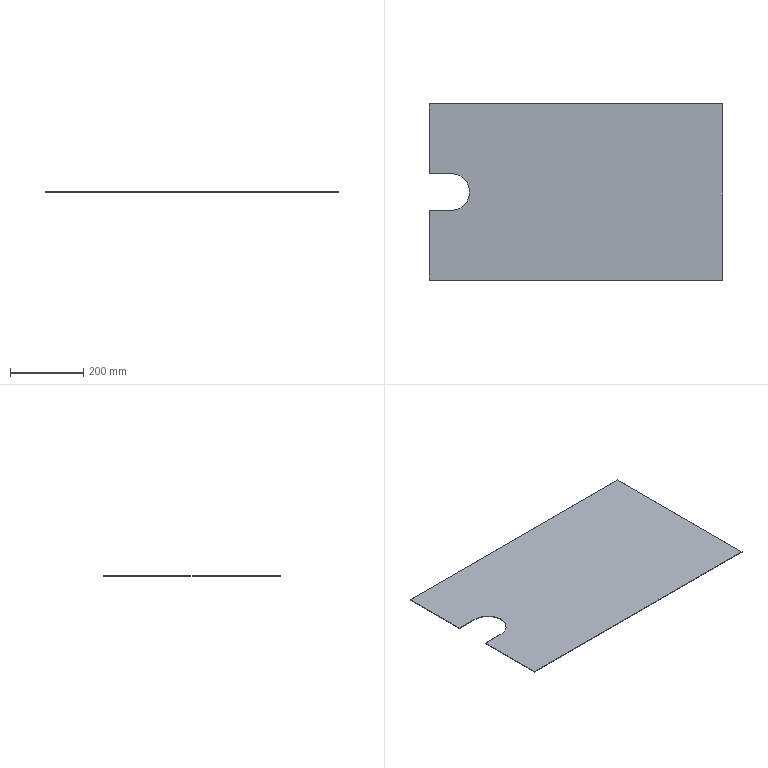Part | SolidWorks | features FlatPattern 1, ICE 1, SMBaseFlange 1, SheetMetal 1 | 1 solid | 10 faces | box 800 x 480 x 1.5 mm | volume 561110 mm3 | plane 9 | cylinder 1 | commonest cylinder face diameters 100 x1
STEP:
#1=CARTESIAN_POINT('',(-585.,-50.,-1.5));
#2=VERTEX_POINT('',#1);
#3=CARTESIAN_POINT('',(-585.,-50.,0.));
#4=VERTEX_POINT('',#3);
#5=CARTESIAN_POINT('',(-585.,-50.,-1.5));
#6=DIRECTION('',(0.,0.,1.));
#7=VECTOR('',#6,1000.);
#8=LINE('',#5,#7);
#9=EDGE_CURVE('',#2,#4,#8,.T.);
#10=ORIENTED_EDGE('',*,*,#9,.F.);
#11=CARTESIAN_POINT('',(-585.,-240.,-1.5));
#12=VERTEX_POINT('',#11);
#13=CARTESIAN_POINT('',(-585.,240.,-1.5));
#14=DIRECTION('',(0.,-1.,0.));
#15=VECTOR('',#14,1000.);
#16=LINE('',#13,#15);
#17=EDGE_CURVE('',#2,#12,#16,.T.);
#18=ORIENTED_EDGE('',*,*,#17,.T.);
#19=CARTESIAN_POINT('',(-585.,-240.,0.));
#20=VERTEX_POINT('',#19);
#21=CARTESIAN_POINT('',(-585.,-240.,-1.5));
#22=DIRECTION('',(0.,0.,1.));
#23=VECTOR('',#22,1000.);
#24=LINE('',#21,#23);
#25=EDGE_CURVE('',#12,#20,#24,.T.);
#26=ORIENTED_EDGE('',*,*,#25,.T.);
#27=CARTESIAN_POINT('',(-585.,240.,0.));
#28=DIRECTION('',(0.,-1.,0.));
#29=VECTOR('',#28,1000.);
#30=LINE('',#27,#29);
#31=EDGE_CURVE('',#4,#20,#30,.T.);
#32=ORIENTED_EDGE('',*,*,#31,.F.);
#33=EDGE_LOOP('',(#10,#18,#26,#32));
#34=FACE_OUTER_BOUND('',#33,.T.);
#35=CARTESIAN_POINT('',(-585.,240.,-1.5));
#36=DIRECTION('',(-1.,0.,0.));
#37=DIRECTION('',(0.,0.,1.));
#38=AXIS2_PLACEMENT_3D('',#35,#36,#37);
#39=PLANE('',#38);
#40=ADVANCED_FACE('',(#34),#39,.T.);
#41=CARTESIAN_POINT('',(215.,-240.,0.));
#42=VERTEX_POINT('',#41);
#43=CARTESIAN_POINT('',(215.,240.,0.));
#44=VERTEX_POINT('',#43);
#45=CARTESIAN_POINT('',(215.,240.,0.));
#46=DIRECTION('',(0.,1.,0.));
#47=VECTOR('',#46,1000.);
#48=LINE('',#45,#47);
#49=EDGE_CURVE('',#42,#44,#48,.T.);
#50=ORIENTED_EDGE('',*,*,#49,.F.);
#51=CARTESIAN_POINT('',(215.,-240.,-1.5));
#52=VERTEX_POINT('',#51);
#53=CARTESIAN_POINT('',(215.,-240.,-1.5));
#54=DIRECTION('',(0.,0.,1.));
#55=VECTOR('',#54,1000.);
#56=LINE('',#53,#55);
#57=EDGE_CURVE('',#52,#42,#56,.T.);
#58=ORIENTED_EDGE('',*,*,#57,.F.);
#59=CARTESIAN_POINT('',(215.,240.,-1.5));
#60=VERTEX_POINT('',#59);
#61=CARTESIAN_POINT('',(215.,240.,-1.5));
#62=DIRECTION('',(0.,1.,0.));
#63=VECTOR('',#62,1000.);
#64=LINE('',#61,#63);
#65=EDGE_CURVE('',#52,#60,#64,.T.);
#66=ORIENTED_EDGE('',*,*,#65,.T.);
#67=CARTESIAN_POINT('',(215.,240.,-1.5));
#68=DIRECTION('',(0.,0.,1.));
#69=VECTOR('',#68,1000.);
#70=LINE('',#67,#69);
#71=EDGE_CURVE('',#60,#44,#70,.T.);
#72=ORIENTED_EDGE('',*,*,#71,.T.);
#73=EDGE_LOOP('',(#50,#58,#66,#72));
#74=FACE_OUTER_BOUND('',#73,.T.);
#75=CARTESIAN_POINT('',(215.,240.,-1.5));
#76=DIRECTION('',(1.,0.,0.));
#77=DIRECTION('',(0.,0.,-1.));
#78=AXIS2_PLACEMENT_3D('',#75,#76,#77);
#79=PLANE('',#78);
#80=ADVANCED_FACE('',(#74),#79,.T.);
#81=CARTESIAN_POINT('',(-585.,-240.,0.));
#82=DIRECTION('',(1.,0.,0.));
#83=VECTOR('',#82,1000.);
#84=LINE('',#81,#83);
#85=EDGE_CURVE('',#20,#42,#84,.T.);
#86=ORIENTED_EDGE('',*,*,#85,.F.);
#87=ORIENTED_EDGE('',*,*,#25,.F.);
#88=CARTESIAN_POINT('',(-585.,-240.,-1.5));
#89=DIRECTION('',(1.,0.,0.));
#90=VECTOR('',#89,1000.);
#91=LINE('',#88,#90);
#92=EDGE_CURVE('',#12,#52,#91,.T.);
#93=ORIENTED_EDGE('',*,*,#92,.T.);
#94=ORIENTED_EDGE('',*,*,#57,.T.);
#95=EDGE_LOOP('',(#86,#87,#93,#94));
#96=FACE_OUTER_BOUND('',#95,.T.);
#97=CARTESIAN_POINT('',(-585.,-240.,-1.5));
#98=DIRECTION('',(0.,-1.,0.));
#99=DIRECTION('',(0.,0.,-1.));
#100=AXIS2_PLACEMENT_3D('',#97,#98,#99);
#101=PLANE('',#100);
#102=ADVANCED_FACE('',(#96),#101,.T.);
#103=CARTESIAN_POINT('',(-585.,50.,0.));
#104=VERTEX_POINT('',#103);
#105=CARTESIAN_POINT('',(-585.,50.,-1.5));
#106=VERTEX_POINT('',#105);
#107=CARTESIAN_POINT('',(-585.,50.,-1.5));
#108=DIRECTION('',(0.,0.,-1.));
#109=VECTOR('',#108,1000.);
#110=LINE('',#107,#109);
#111=EDGE_CURVE('',#104,#106,#110,.T.);
#112=ORIENTED_EDGE('',*,*,#111,.F.);
#113=CARTESIAN_POINT('',(-585.,240.,0.));
#114=VERTEX_POINT('',#113);
#115=CARTESIAN_POINT('',(-585.,240.,0.));
#116=DIRECTION('',(0.,-1.,0.));
#117=VECTOR('',#116,1000.);
#118=LINE('',#115,#117);
#119=EDGE_CURVE('',#114,#104,#118,.T.);
#120=ORIENTED_EDGE('',*,*,#119,.F.);
#121=CARTESIAN_POINT('',(-585.,240.,-1.5));
#122=VERTEX_POINT('',#121);
#123=CARTESIAN_POINT('',(-585.,240.,-1.5));
#124=DIRECTION('',(0.,0.,1.));
#125=VECTOR('',#124,1000.);
#126=LINE('',#123,#125);
#127=EDGE_CURVE('',#122,#114,#126,.T.);
#128=ORIENTED_EDGE('',*,*,#127,.F.);
#129=CARTESIAN_POINT('',(-585.,240.,-1.5));
#130=DIRECTION('',(0.,-1.,0.));
#131=VECTOR('',#130,1000.);
#132=LINE('',#129,#131);
#133=EDGE_CURVE('',#122,#106,#132,.T.);
#134=ORIENTED_EDGE('',*,*,#133,.T.);
#135=EDGE_LOOP('',(#112,#120,#128,#134));
#136=FACE_OUTER_BOUND('',#135,.T.);
#137=CARTESIAN_POINT('',(-585.,240.,-1.5));
#138=DIRECTION('',(-1.,0.,0.));
#139=DIRECTION('',(0.,0.,1.));
#140=AXIS2_PLACEMENT_3D('',#137,#138,#139);
#141=PLANE('',#140);
#142=ADVANCED_FACE('',(#136),#141,.T.);
#143=CARTESIAN_POINT('',(-585.,240.,0.));
#144=DIRECTION('',(-1.,0.,0.));
#145=VECTOR('',#144,1000.);
#146=LINE('',#143,#145);
#147=EDGE_CURVE('',#44,#114,#146,.T.);
#148=ORIENTED_EDGE('',*,*,#147,.F.);
#149=ORIENTED_EDGE('',*,*,#71,.F.);
#150=CARTESIAN_POINT('',(-585.,240.,-1.5));
#151=DIRECTION('',(-1.,0.,0.));
#152=VECTOR('',#151,1000.);
#153=LINE('',#150,#152);
#154=EDGE_CURVE('',#60,#122,#153,.T.);
#155=ORIENTED_EDGE('',*,*,#154,.T.);
#156=ORIENTED_EDGE('',*,*,#127,.T.);
#157=EDGE_LOOP('',(#148,#149,#155,#156));
#158=FACE_OUTER_BOUND('',#157,.T.);
#159=CARTESIAN_POINT('',(-585.,240.,-1.5));
#160=DIRECTION('',(0.,1.,0.));
#161=DIRECTION('',(0.,0.,1.));
#162=AXIS2_PLACEMENT_3D('',#159,#160,#161);
#163=PLANE('',#162);
#164=ADVANCED_FACE('',(#158),#163,.T.);
#165=ORIENTED_EDGE('',*,*,#17,.F.);
#166=CARTESIAN_POINT('',(-525.,-50.,-1.5));
#167=VERTEX_POINT('',#166);
#168=CARTESIAN_POINT('',(0.,-50.,-1.5));
#169=DIRECTION('',(1.,0.,0.));
#170=VECTOR('',#169,1000.);
#171=LINE('',#168,#170);
#172=EDGE_CURVE('',#2,#167,#171,.T.);
#173=ORIENTED_EDGE('',*,*,#172,.T.);
#174=CARTESIAN_POINT('',(-525.,50.,-1.5));
#175=VERTEX_POINT('',#174);
#176=CARTESIAN_POINT('',(-525.,0.,-1.5));
#177=DIRECTION('',(0.,0.,1.));
#178=DIRECTION('',(1.,0.,0.));
#179=AXIS2_PLACEMENT_3D('',#176,#177,#178);
#180=CIRCLE('',#179,50.);
#181=EDGE_CURVE('',#167,#175,#180,.T.);
#182=ORIENTED_EDGE('',*,*,#181,.T.);
#183=CARTESIAN_POINT('',(0.,50.,-1.5));
#184=DIRECTION('',(-1.,0.,0.));
#185=VECTOR('',#184,1000.);
#186=LINE('',#183,#185);
#187=EDGE_CURVE('',#175,#106,#186,.T.);
#188=ORIENTED_EDGE('',*,*,#187,.T.);
#189=ORIENTED_EDGE('',*,*,#133,.F.);
#190=ORIENTED_EDGE('',*,*,#154,.F.);
#191=ORIENTED_EDGE('',*,*,#65,.F.);
#192=ORIENTED_EDGE('',*,*,#92,.F.);
#193=EDGE_LOOP('',(#165,#173,#182,#188,#189,#190,#191,#192));
#194=FACE_OUTER_BOUND('',#193,.T.);
#195=CARTESIAN_POINT('',(0.,0.,-1.5));
#196=DIRECTION('',(0.,0.,1.));
#197=DIRECTION('',(1.,0.,0.));
#198=AXIS2_PLACEMENT_3D('',#195,#196,#197);
#199=PLANE('',#198);
#200=ADVANCED_FACE('',(#194),#199,.F.);
#201=CARTESIAN_POINT('',(-525.,-50.,0.));
#202=VERTEX_POINT('',#201);
#203=CARTESIAN_POINT('',(0.,-50.,0.));
#204=DIRECTION('',(1.,0.,0.));
#205=VECTOR('',#204,1000.);
#206=LINE('',#203,#205);
#207=EDGE_CURVE('',#4,#202,#206,.T.);
#208=ORIENTED_EDGE('',*,*,#207,.F.);
#209=ORIENTED_EDGE('',*,*,#31,.T.);
#210=ORIENTED_EDGE('',*,*,#85,.T.);
#211=ORIENTED_EDGE('',*,*,#49,.T.);
#212=ORIENTED_EDGE('',*,*,#147,.T.);
#213=ORIENTED_EDGE('',*,*,#119,.T.);
#214=CARTESIAN_POINT('',(-525.,50.,0.));
#215=VERTEX_POINT('',#214);
#216=CARTESIAN_POINT('',(0.,50.,0.));
#217=DIRECTION('',(-1.,0.,0.));
#218=VECTOR('',#217,1000.);
#219=LINE('',#216,#218);
#220=EDGE_CURVE('',#215,#104,#219,.T.);
#221=ORIENTED_EDGE('',*,*,#220,.F.);
#222=CARTESIAN_POINT('',(-525.,0.,0.));
#223=DIRECTION('',(0.,0.,1.));
#224=DIRECTION('',(1.,0.,0.));
#225=AXIS2_PLACEMENT_3D('',#222,#223,#224);
#226=CIRCLE('',#225,50.);
#227=EDGE_CURVE('',#202,#215,#226,.T.);
#228=ORIENTED_EDGE('',*,*,#227,.F.);
#229=EDGE_LOOP('',(#208,#209,#210,#211,#212,#213,#221,#228));
#230=FACE_OUTER_BOUND('',#229,.T.);
#231=CARTESIAN_POINT('',(0.,0.,0.));
#232=DIRECTION('',(0.,0.,1.));
#233=DIRECTION('',(1.,0.,0.));
#234=AXIS2_PLACEMENT_3D('',#231,#232,#233);
#235=PLANE('',#234);
#236=ADVANCED_FACE('',(#230),#235,.T.);
#237=ORIENTED_EDGE('',*,*,#9,.T.);
#238=ORIENTED_EDGE('',*,*,#207,.T.);
#239=CARTESIAN_POINT('',(-525.,-50.,0.5));
#240=DIRECTION('',(0.,0.,-1.));
#241=VECTOR('',#240,1000.);
#242=LINE('',#239,#241);
#243=EDGE_CURVE('',#202,#167,#242,.T.);
#244=ORIENTED_EDGE('',*,*,#243,.T.);
#245=ORIENTED_EDGE('',*,*,#172,.F.);
#246=EDGE_LOOP('',(#237,#238,#244,#245));
#247=FACE_OUTER_BOUND('',#246,.T.);
#248=CARTESIAN_POINT('',(-525.,-50.,0.5));
#249=DIRECTION('',(0.,-1.,0.));
#250=DIRECTION('',(0.,0.,-1.));
#251=AXIS2_PLACEMENT_3D('',#248,#249,#250);
#252=PLANE('',#251);
#253=ADVANCED_FACE('',(#247),#252,.F.);
#254=ORIENTED_EDGE('',*,*,#243,.F.);
#255=ORIENTED_EDGE('',*,*,#227,.T.);
#256=CARTESIAN_POINT('',(-525.,50.,0.5));
#257=DIRECTION('',(0.,0.,-1.));
#258=VECTOR('',#257,1000.);
#259=LINE('',#256,#258);
#260=EDGE_CURVE('',#215,#175,#259,.T.);
#261=ORIENTED_EDGE('',*,*,#260,.T.);
#262=ORIENTED_EDGE('',*,*,#181,.F.);
#263=EDGE_LOOP('',(#254,#255,#261,#262));
#264=FACE_OUTER_BOUND('',#263,.T.);
#265=CARTESIAN_POINT('',(-525.,0.,0.5));
#266=DIRECTION('',(0.,0.,-1.));
#267=DIRECTION('',(-1.,0.,0.));
#268=AXIS2_PLACEMENT_3D('',#265,#266,#267);
#269=CYLINDRICAL_SURFACE('',#268,50.);
#270=ADVANCED_FACE('',(#264),#269,.F.);
#271=ORIENTED_EDGE('',*,*,#260,.F.);
#272=ORIENTED_EDGE('',*,*,#220,.T.);
#273=ORIENTED_EDGE('',*,*,#111,.T.);
#274=ORIENTED_EDGE('',*,*,#187,.F.);
#275=EDGE_LOOP('',(#271,#272,#273,#274));
#276=FACE_OUTER_BOUND('',#275,.T.);
#277=CARTESIAN_POINT('',(-525.,50.,0.5));
#278=DIRECTION('',(0.,1.,0.));
#279=DIRECTION('',(0.,0.,1.));
#280=AXIS2_PLACEMENT_3D('',#277,#278,#279);
#281=PLANE('',#280);
#282=ADVANCED_FACE('',(#276),#281,.F.);
#283=CLOSED_SHELL('',(#40,#80,#102,#142,#164,#200,#236,#253,#270,#282));
#284=MANIFOLD_SOLID_BREP('',#283);
#285=CARTESIAN_POINT('',(0.,0.,0.));
#286=DIRECTION('',(0.,0.,1.));
#287=DIRECTION('',(1.,0.,0.));
#288=AXIS2_PLACEMENT_3D('',#285,#286,#287);
#289=(LENGTH_UNIT()NAMED_UNIT(*)SI_UNIT(.MILLI.,.METRE.));
#290=UNCERTAINTY_MEASURE_WITH_UNIT(LENGTH_MEASURE(0.00001),#289,'','');
#291=(NAMED_UNIT(*)PLANE_ANGLE_UNIT()SI_UNIT($,.RADIAN.));
#292=(NAMED_UNIT(*)SI_UNIT($,.STERADIAN.)SOLID_ANGLE_UNIT());
#293=(GEOMETRIC_REPRESENTATION_CONTEXT(3)GLOBAL_UNCERTAINTY_ASSIGNED_CONTEXT((#290))GLOBAL_UNIT_ASSIGNED_CONTEXT((#289,#291,#292))REPRESENTATION_CONTEXT('',''));
#294=ADVANCED_BREP_SHAPE_REPRESENTATION('',(#284,#288),#293);